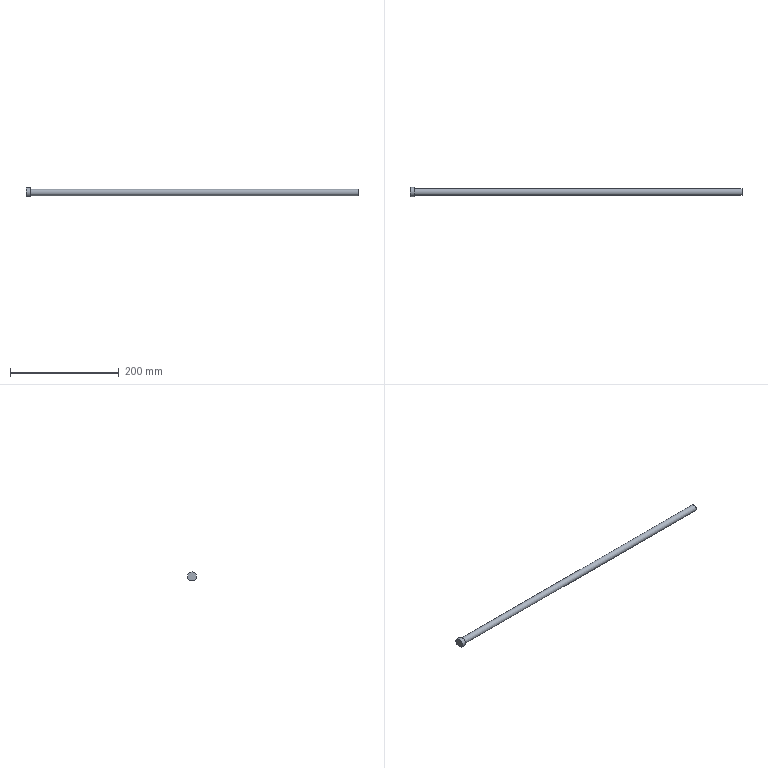Part | STEP file | solid 47 | 1 solid | 6 faces | box 610 x 17 x 15 mm | volume 69781 mm3 | plane 4 | cylinder 2 | commonest cylinder face diameters 12 x1 17 x1